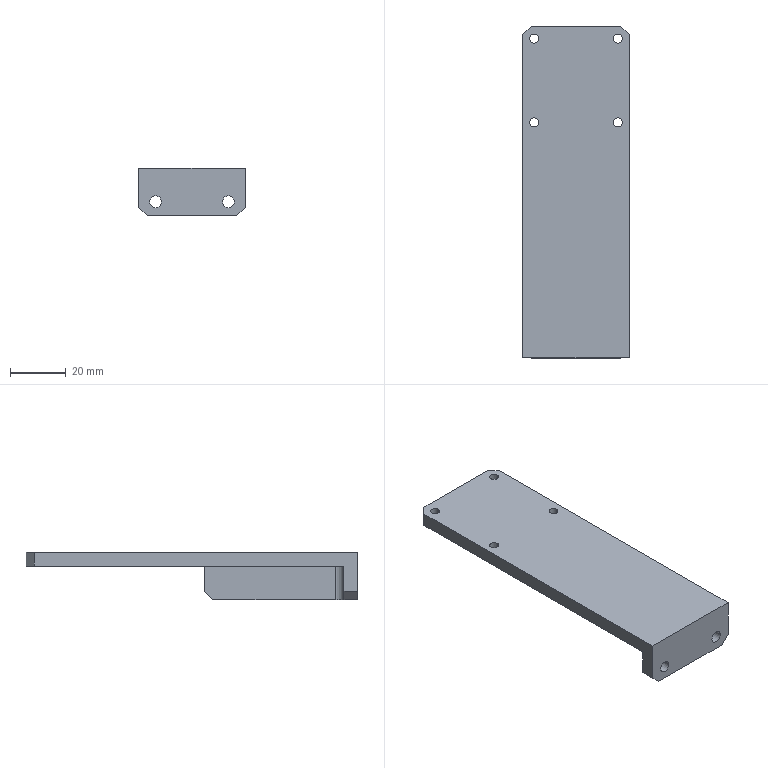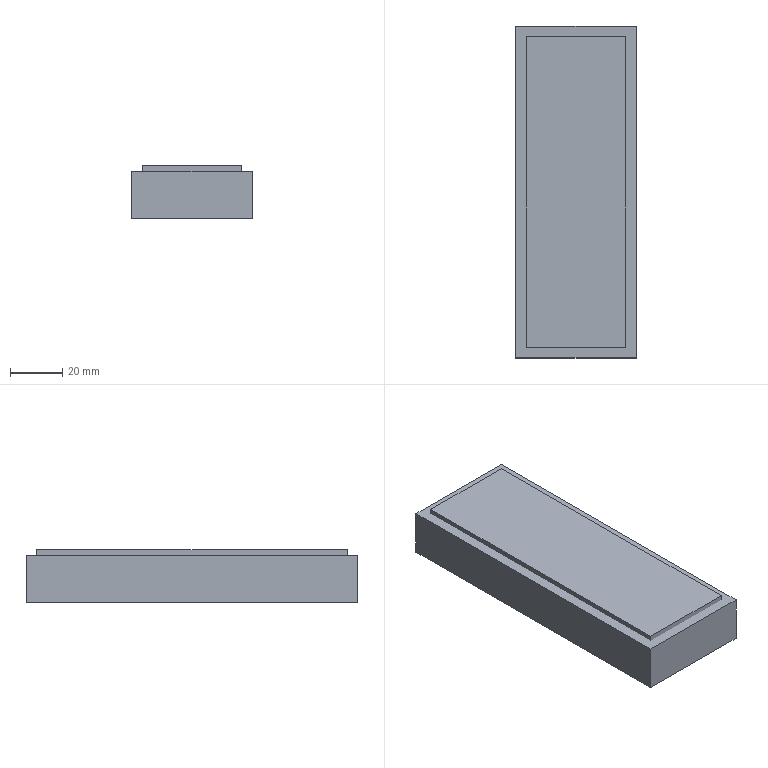CAM job | NX | 3-axis milling, drilling | part box 38.1 x 118.8 x 17 mm | stock box 46.1 x 126.8 x 20 mm
Tools:
number,name,description,diameter,corner_radius,flute_length,length,flutes
19,D80,Milling Tool-5 Parameters,80.0,0.0,50.0,75.0,2
1,D6A45,Milling Tool-5 Parameters,6.0,0.0,50.0,75.0,2
3,3.2ZT,Drilling Tool,3.2,0.0,35.0,50.0,2
15,D10,Milling Tool-5 Parameters,10.0,0.0,50.0,75.0,2
14,D10JING,Milling Tool-5 Parameters,10.0,0.0,50.0,75.0,2
12,D6,Milling Tool-5 Parameters,6.0,0.0,50.0,75.0,2
16,D6R0.5,Milling Tool-5 Parameters,6.0,0.5,50.0,75.0,2
Operations:
program,operation,operation_type,tool,method,geometry_group,spindle_rpm,surface_speed,feed_per_tooth,feed_cut,feed_plunge,cut_length_mm,path_length_mm,cut_time_min,machine_time_min
1,FLOOR_WALL_COPY,VolumeBased25DMillingOperation,D80,METHOD,A,6500.0,1633.0,0.1154,1500.0,100.0,222.8,276.8,0.1485,0.1539
1,DRILLING_COPY_1,Operation,D6A45,METHOD,A,5000.0,94.0,0.035,350.0,0.0,16.0,191.449,0.0457,0.0633
1,DRILLING_COPY_1_COPY_1,Operation,3.2ZT,METHOD,A,2000.0,21.0,0.045,180.0,0.0,41.846,243.14,0.2325,0.2526
1,ADAPTIVE_MILLING,CavityMilling,D10,METHOD,A,9500.0,298.0,0.1579,3000.0,1000.0,1421.61,1509.61,0.4759,0.4847
1,ZLEVEL_PROFILE_COPY_1_COPY_COPY_1,ZLevelMilling,D10JING,METHOD,A,9500.0,298.0,0.0632,1200.0,1000.0,349.04,441.04,0.2915,0.3007
1,PLANAR_MILL_COPY_COPY_COPY_COPY_COPY_COPY_1_COPY_1,PlanarMilling,D6A45,METHOD,A,9500.0,179.0,0.0658,1250.0,100.0,354.816,779.184,0.2839,0.3263
2,FLOOR_WALL_COPY_COPY,VolumeBased25DMillingOperation,D80,METHOD,B,6500.0,1633.0,0.1154,1500.0,100.0,644.4,1218.001,0.4296,0.487
2,FLOOR_WALL,VolumeBased25DMillingOperation,D10,METHOD,B,9500.0,298.0,0.1579,3000.0,1000.0,9187.459,9392.036,3.081,3.102
2,FLOOR_WALL_COPY_1,VolumeBased25DMillingOperation,D10JING,METHOD,B,9500.0,298.0,0.0632,1200.0,1000.0,1025.072,1181.337,0.8562,0.8718
2,ZLEVEL_PROFILE,ZLevelMilling,D6,METHOD,B,9500.0,179.0,0.0842,1600.0,100.0,352.703,636.354,0.2204,0.2488
2,PLANAR_MILL_COPY_COPY_COPY_COPY_COPY_COPY_1_COPY_1_COPY,PlanarMilling,D6A45,METHOD,B,9500.0,179.0,0.0658,1250.0,100.0,313.2,936.79,0.2506,0.3129
2,PLANAR_MILL_COPY_COPY_COPY_COPY_COPY_COPY_1_COPY_1_COPY_COPY,PlanarMilling,D6A45,METHOD,B,9500.0,179.0,0.0658,1250.0,100.0,195.733,254.733,0.1566,0.1625
2,ZLEVEL_PROFILE_1,ZLevelMilling,D6R0.5,METHOD,B,9500.0,119.0,0.1842,3500.0,100.0,1076.536,1348.465,0.3076,0.3348